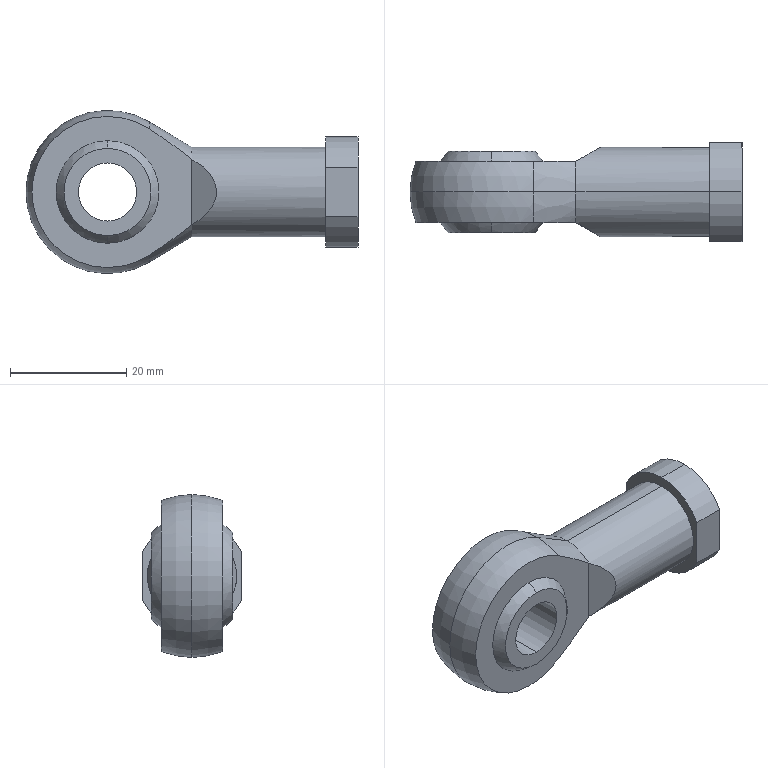Part | SolidWorks | features Draft 2, HoleWzd 2, ICE 2, BaseBody 1, Chamfer 1 | 1 solid | 32 faces | box 57 x 17 x 28 mm | volume 10383 mm3 | plane 10 | cylinder 9 | cone 7 | sphere 6 | commonest cylinder face diameters 19 x3 8.376 x2 10 x2 15.352 x2
STEP:
#1=CARTESIAN_POINT('',(42.188,0.,4.188));
#2=VERTEX_POINT('',#1);
#3=CARTESIAN_POINT('',(42.188,0.,-4.188));
#4=VERTEX_POINT('',#3);
#5=CARTESIAN_POINT('',(42.188,0.,0.));
#6=DIRECTION('',(1.,0.,0.));
#7=DIRECTION('',(0.,0.,1.));
#8=AXIS2_PLACEMENT_3D('',#5,#6,#7);
#9=CIRCLE('',#8,4.188);
#10=EDGE_CURVE('',#2,#4,#9,.T.);
#11=ORIENTED_EDGE('',*,*,#10,.F.);
#12=CARTESIAN_POINT('',(43.,0.,5.));
#13=VERTEX_POINT('',#12);
#14=CARTESIAN_POINT('',(42.188,0.,4.188));
#15=DIRECTION('',(0.7071,0.,0.7071));
#16=VECTOR('',#15,1000.);
#17=LINE('',#14,#16);
#18=EDGE_CURVE('',#2,#13,#17,.T.);
#19=ORIENTED_EDGE('',*,*,#18,.T.);
#20=CARTESIAN_POINT('',(43.,0.,-5.));
#21=VERTEX_POINT('',#20);
#22=CARTESIAN_POINT('',(43.,0.,0.));
#23=DIRECTION('',(-1.,0.,0.));
#24=DIRECTION('',(0.,0.,1.));
#25=AXIS2_PLACEMENT_3D('',#22,#23,#24);
#26=CIRCLE('',#25,5.);
#27=EDGE_CURVE('',#21,#13,#26,.T.);
#28=ORIENTED_EDGE('',*,*,#27,.F.);
#29=CARTESIAN_POINT('',(42.188,0.,-4.188));
#30=DIRECTION('',(0.7071,0.,-0.7071));
#31=VECTOR('',#30,1000.);
#32=LINE('',#29,#31);
#33=EDGE_CURVE('',#4,#21,#32,.T.);
#34=ORIENTED_EDGE('',*,*,#33,.F.);
#35=EDGE_LOOP('',(#11,#19,#28,#34));
#36=FACE_OUTER_BOUND('',#35,.T.);
#37=CARTESIAN_POINT('',(42.188,0.,0.));
#38=DIRECTION('',(1.,0.,0.));
#39=DIRECTION('',(0.,0.,-1.));
#40=AXIS2_PLACEMENT_3D('',#37,#38,#39);
#41=CONICAL_SURFACE('',#40,4.188,0.7854);
#42=ADVANCED_FACE('',(#36),#41,.F.);
#43=CARTESIAN_POINT('',(18.,0.,4.188));
#44=VERTEX_POINT('',#43);
#45=CARTESIAN_POINT('',(18.,0.,-4.188));
#46=VERTEX_POINT('',#45);
#47=CARTESIAN_POINT('',(18.,0.,0.));
#48=DIRECTION('',(1.,0.,0.));
#49=DIRECTION('',(0.,0.,-1.));
#50=AXIS2_PLACEMENT_3D('',#47,#48,#49);
#51=CIRCLE('',#50,4.188);
#52=EDGE_CURVE('',#44,#46,#51,.T.);
#53=ORIENTED_EDGE('',*,*,#52,.F.);
#54=CARTESIAN_POINT('',(43.,0.,4.188));
#55=DIRECTION('',(1.,0.,0.));
#56=VECTOR('',#55,1000.);
#57=LINE('',#54,#56);
#58=EDGE_CURVE('',#44,#2,#57,.T.);
#59=ORIENTED_EDGE('',*,*,#58,.T.);
#60=ORIENTED_EDGE('',*,*,#10,.T.);
#61=CARTESIAN_POINT('',(43.,0.,-4.188));
#62=DIRECTION('',(1.,0.,0.));
#63=VECTOR('',#62,1000.);
#64=LINE('',#61,#63);
#65=EDGE_CURVE('',#46,#4,#64,.T.);
#66=ORIENTED_EDGE('',*,*,#65,.F.);
#67=EDGE_LOOP('',(#53,#59,#60,#66));
#68=FACE_OUTER_BOUND('',#67,.T.);
#69=CARTESIAN_POINT('',(43.,0.,0.));
#70=DIRECTION('',(1.,0.,0.));
#71=DIRECTION('',(0.,0.,-1.));
#72=AXIS2_PLACEMENT_3D('',#69,#70,#71);
#73=CYLINDRICAL_SURFACE('',#72,4.188);
#74=ADVANCED_FACE('',(#68),#73,.F.);
#75=CARTESIAN_POINT('',(15.582,0.,0.));
#76=VERTEX_POINT('',#75);
#77=CARTESIAN_POINT('',(18.,0.,-4.188));
#78=DIRECTION('',(0.5,0.,-0.866));
#79=VECTOR('',#78,1000.);
#80=LINE('',#77,#79);
#81=EDGE_CURVE('',#76,#46,#80,.T.);
#82=ORIENTED_EDGE('',*,*,#81,.F.);
#83=CARTESIAN_POINT('',(18.,0.,4.188));
#84=DIRECTION('',(0.5,0.,0.866));
#85=VECTOR('',#84,1000.);
#86=LINE('',#83,#85);
#87=EDGE_CURVE('',#76,#44,#86,.T.);
#88=ORIENTED_EDGE('',*,*,#87,.T.);
#89=ORIENTED_EDGE('',*,*,#52,.T.);
#90=EDGE_LOOP('',(#82,#88,#89));
#91=FACE_OUTER_BOUND('',#90,.T.);
#92=CARTESIAN_POINT('',(18.,0.,0.));
#93=DIRECTION('',(1.,0.,0.));
#94=DIRECTION('',(0.,0.,-1.));
#95=AXIS2_PLACEMENT_3D('',#92,#93,#94);
#96=CONICAL_SURFACE('',#95,4.188,1.047);
#97=ADVANCED_FACE('',(#91),#96,.F.);
#98=CARTESIAN_POINT('',(0.,7.,-5.));
#99=VERTEX_POINT('',#98);
#100=CARTESIAN_POINT('',(0.,7.,5.));
#101=VERTEX_POINT('',#100);
#102=CARTESIAN_POINT('',(0.,7.,0.));
#103=DIRECTION('',(0.,1.,0.));
#104=DIRECTION('',(0.,0.,1.));
#105=AXIS2_PLACEMENT_3D('',#102,#103,#104);
#106=CIRCLE('',#105,5.);
#107=EDGE_CURVE('',#99,#101,#106,.T.);
#108=ORIENTED_EDGE('',*,*,#107,.T.);
#109=CARTESIAN_POINT('',(0.,-7.,5.));
#110=VERTEX_POINT('',#109);
#111=CARTESIAN_POINT('',(0.,-7.,5.));
#112=DIRECTION('',(0.,-1.,0.));
#113=VECTOR('',#112,1000.);
#114=LINE('',#111,#113);
#115=EDGE_CURVE('',#101,#110,#114,.T.);
#116=ORIENTED_EDGE('',*,*,#115,.T.);
#117=CARTESIAN_POINT('',(0.,-7.,-5.));
#118=VERTEX_POINT('',#117);
#119=CARTESIAN_POINT('',(0.,-7.,0.));
#120=DIRECTION('',(0.,-1.,0.));
#121=DIRECTION('',(0.,0.,-1.));
#122=AXIS2_PLACEMENT_3D('',#119,#120,#121);
#123=CIRCLE('',#122,5.);
#124=EDGE_CURVE('',#110,#118,#123,.T.);
#125=ORIENTED_EDGE('',*,*,#124,.T.);
#126=CARTESIAN_POINT('',(0.,-7.,-5.));
#127=DIRECTION('',(0.,-1.,0.));
#128=VECTOR('',#127,1000.);
#129=LINE('',#126,#128);
#130=EDGE_CURVE('',#99,#118,#129,.T.);
#131=ORIENTED_EDGE('',*,*,#130,.F.);
#132=EDGE_LOOP('',(#108,#116,#125,#131));
#133=FACE_OUTER_BOUND('',#132,.T.);
#134=CARTESIAN_POINT('',(0.,-7.,0.));
#135=DIRECTION('',(0.,-1.,0.));
#136=DIRECTION('',(0.,0.,-1.));
#137=AXIS2_PLACEMENT_3D('',#134,#135,#136);
#138=CYLINDRICAL_SURFACE('',#137,5.);
#139=ADVANCED_FACE('',(#133),#138,.F.);
#140=CARTESIAN_POINT('',(43.,-8.5,4.243));
#141=VERTEX_POINT('',#140);
#142=CARTESIAN_POINT('',(43.,0.,9.5));
#143=VERTEX_POINT('',#142);
#144=CARTESIAN_POINT('',(43.,0.,0.));
#145=DIRECTION('',(-1.,0.,0.));
#146=DIRECTION('',(0.,0.,1.));
#147=AXIS2_PLACEMENT_3D('',#144,#145,#146);
#148=CIRCLE('',#147,9.5);
#149=EDGE_CURVE('',#141,#143,#148,.T.);
#150=ORIENTED_EDGE('',*,*,#149,.T.);
#151=CARTESIAN_POINT('',(37.453,0.,9.5));
#152=VERTEX_POINT('',#151);
#153=CARTESIAN_POINT('',(43.,0.,9.5));
#154=DIRECTION('',(-1.,0.,0.));
#155=VECTOR('',#154,1000.);
#156=LINE('',#153,#155);
#157=EDGE_CURVE('',#143,#152,#156,.T.);
#158=ORIENTED_EDGE('',*,*,#157,.T.);
#159=CARTESIAN_POINT('',(37.453,-8.5,4.243));
#160=VERTEX_POINT('',#159);
#161=CARTESIAN_POINT('',(37.453,0.,0.));
#162=DIRECTION('',(-1.,0.,0.));
#163=DIRECTION('',(0.,0.,1.));
#164=AXIS2_PLACEMENT_3D('',#161,#162,#163);
#165=CIRCLE('',#164,9.5);
#166=EDGE_CURVE('',#160,#152,#165,.T.);
#167=ORIENTED_EDGE('',*,*,#166,.F.);
#168=CARTESIAN_POINT('',(43.,-8.5,4.243));
#169=DIRECTION('',(-1.,0.,0.));
#170=VECTOR('',#169,1000.);
#171=LINE('',#168,#170);
#172=EDGE_CURVE('',#141,#160,#171,.T.);
#173=ORIENTED_EDGE('',*,*,#172,.F.);
#174=EDGE_LOOP('',(#150,#158,#167,#173));
#175=FACE_OUTER_BOUND('',#174,.T.);
#176=CARTESIAN_POINT('',(43.,0.,0.));
#177=DIRECTION('',(-1.,0.,0.));
#178=DIRECTION('',(0.,0.,1.));
#179=AXIS2_PLACEMENT_3D('',#176,#177,#178);
#180=CYLINDRICAL_SURFACE('',#179,9.5);
#181=ADVANCED_FACE('',(#175),#180,.T.);
#182=CARTESIAN_POINT('',(37.453,0.,-7.676));
#183=VERTEX_POINT('',#182);
#184=CARTESIAN_POINT('',(37.453,0.,7.676));
#185=VERTEX_POINT('',#184);
#186=CARTESIAN_POINT('',(37.453,0.,0.));
#187=DIRECTION('',(1.,0.,0.));
#188=DIRECTION('',(0.,0.,-1.));
#189=AXIS2_PLACEMENT_3D('',#186,#187,#188);
#190=CIRCLE('',#189,7.676);
#191=EDGE_CURVE('',#183,#185,#190,.T.);
#192=ORIENTED_EDGE('',*,*,#191,.F.);
#193=CARTESIAN_POINT('',(14.491,0.,-7.676));
#194=VERTEX_POINT('',#193);
#195=CARTESIAN_POINT('',(37.453,0.,-7.676));
#196=DIRECTION('',(-1.,0.,0.));
#197=VECTOR('',#196,1000.);
#198=LINE('',#195,#197);
#199=EDGE_CURVE('',#183,#194,#198,.T.);
#200=ORIENTED_EDGE('',*,*,#199,.T.);
#201=CARTESIAN_POINT('',(14.491,5.25,-5.6));
#202=VERTEX_POINT('',#201);
#203=CARTESIAN_POINT('',(14.491,0.,0.));
#204=DIRECTION('',(1.,0.,0.));
#205=DIRECTION('',(0.,0.,1.));
#206=AXIS2_PLACEMENT_3D('',#203,#204,#205);
#207=CIRCLE('',#206,7.676);
#208=EDGE_CURVE('',#194,#202,#207,.T.);
#209=ORIENTED_EDGE('',*,*,#208,.T.);
#210=CARTESIAN_POINT('',(14.491,5.25,5.6));
#211=VERTEX_POINT('',#210);
#212=CARTESIAN_POINT('',(14.491,5.25,-5.6));
#213=CARTESIAN_POINT('',(20.468,8.701,-2.365));
#214=CARTESIAN_POINT('',(20.468,8.701,2.365));
#215=CARTESIAN_POINT('',(14.491,5.25,5.6));
#216=(BOUNDED_CURVE()B_SPLINE_CURVE(3,(#212,#213,#214,#215),.UNSPECIFIED.,.F.,.F.)B_SPLINE_CURVE_WITH_KNOTS((4,4),(2.324,3.959),.UNSPECIFIED.)CURVE()GEOMETRIC_REPRESENTATION_ITEM()RATIONAL_B_SPLINE_CURVE((1.,0.7893,0.7893,1.))REPRESENTATION_ITEM(''));
#217=EDGE_CURVE('',#202,#211,#216,.T.);
#218=ORIENTED_EDGE('',*,*,#217,.T.);
#219=CARTESIAN_POINT('',(14.491,0.,7.676));
#220=VERTEX_POINT('',#219);
#221=CARTESIAN_POINT('',(14.491,0.,0.));
#222=DIRECTION('',(1.,0.,0.));
#223=DIRECTION('',(0.,0.,1.));
#224=AXIS2_PLACEMENT_3D('',#221,#222,#223);
#225=CIRCLE('',#224,7.676);
#226=EDGE_CURVE('',#211,#220,#225,.T.);
#227=ORIENTED_EDGE('',*,*,#226,.T.);
#228=CARTESIAN_POINT('',(37.453,0.,7.676));
#229=DIRECTION('',(-1.,0.,0.));
#230=VECTOR('',#229,1000.);
#231=LINE('',#228,#230);
#232=EDGE_CURVE('',#185,#220,#231,.T.);
#233=ORIENTED_EDGE('',*,*,#232,.F.);
#234=EDGE_LOOP('',(#192,#200,#209,#218,#227,#233));
#235=FACE_OUTER_BOUND('',#234,.T.);
#236=CARTESIAN_POINT('',(37.453,0.,0.));
#237=DIRECTION('',(-1.,0.,0.));
#238=DIRECTION('',(0.,0.,1.));
#239=AXIS2_PLACEMENT_3D('',#236,#237,#238);
#240=CYLINDRICAL_SURFACE('',#239,7.676);
#241=ADVANCED_FACE('',(#235),#240,.T.);
#242=CARTESIAN_POINT('',(0.,5.25,-8.813));
#243=VERTEX_POINT('',#242);
#244=CARTESIAN_POINT('',(0.,5.25,8.813));
#245=VERTEX_POINT('',#244);
#246=CARTESIAN_POINT('',(0.,5.25,0.));
#247=DIRECTION('',(0.,1.,0.));
#248=DIRECTION('',(0.,0.,1.));
#249=AXIS2_PLACEMENT_3D('',#246,#247,#248);
#250=CIRCLE('',#249,8.813);
#251=EDGE_CURVE('',#243,#245,#250,.T.);
#252=ORIENTED_EDGE('',*,*,#251,.T.);
#253=CARTESIAN_POINT('',(0.,7.,7.498));
#254=VERTEX_POINT('',#253);
#255=CARTESIAN_POINT('',(0.,0.,0.));
#256=DIRECTION('',(-1.,0.,0.));
#257=DIRECTION('',(0.,0.,1.));
#258=AXIS2_PLACEMENT_3D('',#255,#256,#257);
#259=CIRCLE('',#258,10.258);
#260=EDGE_CURVE('',#245,#254,#259,.T.);
#261=ORIENTED_EDGE('',*,*,#260,.T.);
#262=CARTESIAN_POINT('',(0.,7.,-7.498));
#263=VERTEX_POINT('',#262);
#264=CARTESIAN_POINT('',(0.,7.,0.));
#265=DIRECTION('',(0.,-1.,0.));
#266=DIRECTION('',(0.,0.,1.));
#267=AXIS2_PLACEMENT_3D('',#264,#265,#266);
#268=CIRCLE('',#267,7.498);
#269=EDGE_CURVE('',#254,#263,#268,.T.);
#270=ORIENTED_EDGE('',*,*,#269,.T.);
#271=CARTESIAN_POINT('',(0.,0.,0.));
#272=DIRECTION('',(1.,0.,0.));
#273=DIRECTION('',(0.,1.,0.));
#274=AXIS2_PLACEMENT_3D('',#271,#272,#273);
#275=CIRCLE('',#274,10.258);
#276=EDGE_CURVE('',#243,#263,#275,.T.);
#277=ORIENTED_EDGE('',*,*,#276,.F.);
#278=EDGE_LOOP('',(#252,#261,#270,#277));
#279=FACE_OUTER_BOUND('',#278,.T.);
#280=CARTESIAN_POINT('',(0.,0.,0.));
#281=DIRECTION('',(-1.,0.,0.));
#282=DIRECTION('',(0.,0.5011,-0.8654));
#283=AXIS2_PLACEMENT_3D('',#280,#281,#282);
#284=SPHERICAL_SURFACE('',#283,10.258);
#285=ADVANCED_FACE('',(#279),#284,.T.);
#286=CARTESIAN_POINT('',(0.,-5.25,8.813));
#287=VERTEX_POINT('',#286);
#288=CARTESIAN_POINT('',(0.,-5.25,-8.813));
#289=VERTEX_POINT('',#288);
#290=CARTESIAN_POINT('',(0.,-5.25,0.));
#291=DIRECTION('',(0.,-1.,0.));
#292=DIRECTION('',(0.,0.,-1.));
#293=AXIS2_PLACEMENT_3D('',#290,#291,#292);
#294=CIRCLE('',#293,8.813);
#295=EDGE_CURVE('',#287,#289,#294,.T.);
#296=ORIENTED_EDGE('',*,*,#295,.T.);
#297=CARTESIAN_POINT('',(0.,-7.,-7.498));
#298=VERTEX_POINT('',#297);
#299=CARTESIAN_POINT('',(0.,0.,0.));
#300=DIRECTION('',(-1.,0.,0.));
#301=DIRECTION('',(0.,0.,1.));
#302=AXIS2_PLACEMENT_3D('',#299,#300,#301);
#303=CIRCLE('',#302,10.258);
#304=EDGE_CURVE('',#289,#298,#303,.T.);
#305=ORIENTED_EDGE('',*,*,#304,.T.);
#306=CARTESIAN_POINT('',(0.,-7.,7.498));
#307=VERTEX_POINT('',#306);
#308=CARTESIAN_POINT('',(0.,-7.,0.));
#309=DIRECTION('',(0.,1.,0.));
#310=DIRECTION('',(0.,0.,-1.));
#311=AXIS2_PLACEMENT_3D('',#308,#309,#310);
#312=CIRCLE('',#311,7.498);
#313=EDGE_CURVE('',#298,#307,#312,.T.);
#314=ORIENTED_EDGE('',*,*,#313,.T.);
#315=CARTESIAN_POINT('',(0.,0.,0.));
#316=DIRECTION('',(1.,0.,0.));
#317=DIRECTION('',(0.,1.,0.));
#318=AXIS2_PLACEMENT_3D('',#315,#316,#317);
#319=CIRCLE('',#318,10.258);
#320=EDGE_CURVE('',#287,#307,#319,.T.);
#321=ORIENTED_EDGE('',*,*,#320,.F.);
#322=EDGE_LOOP('',(#296,#305,#314,#321));
#323=FACE_OUTER_BOUND('',#322,.T.);
#324=CARTESIAN_POINT('',(0.,0.,0.));
#325=DIRECTION('',(-1.,0.,0.));
#326=DIRECTION('',(0.,-0.5011,0.8654));
#327=AXIS2_PLACEMENT_3D('',#324,#325,#326);
#328=SPHERICAL_SURFACE('',#327,10.258);
#329=ADVANCED_FACE('',(#323),#328,.T.);
#330=CARTESIAN_POINT('',(14.491,-5.25,5.6));
#331=VERTEX_POINT('',#330);
#332=CARTESIAN_POINT('',(14.491,0.,0.));
#333=DIRECTION('',(1.,0.,0.));
#334=DIRECTION('',(0.,0.,1.));
#335=AXIS2_PLACEMENT_3D('',#332,#333,#334);
#336=CIRCLE('',#335,7.676);
#337=EDGE_CURVE('',#220,#331,#336,.T.);
#338=ORIENTED_EDGE('',*,*,#337,.F.);
#339=CARTESIAN_POINT('',(7.15,0.,12.037));
#340=VERTEX_POINT('',#339);
#341=CARTESIAN_POINT('',(7.15,0.,12.037));
#342=DIRECTION('',(-0.8598,0.,0.5107));
#343=VECTOR('',#342,1000.);
#344=LINE('',#341,#343);
#345=EDGE_CURVE('',#220,#340,#344,.T.);
#346=ORIENTED_EDGE('',*,*,#345,.T.);
#347=CARTESIAN_POINT('',(7.15,-5.25,10.831));
#348=VERTEX_POINT('',#347);
#349=CARTESIAN_POINT('',(7.15,0.,0.));
#350=DIRECTION('',(1.,0.,0.));
#351=DIRECTION('',(0.,0.,1.));
#352=AXIS2_PLACEMENT_3D('',#349,#350,#351);
#353=CIRCLE('',#352,12.037);
#354=EDGE_CURVE('',#340,#348,#353,.T.);
#355=ORIENTED_EDGE('',*,*,#354,.T.);
#356=CARTESIAN_POINT('',(7.15,-5.25,10.831));
#357=CARTESIAN_POINT('',(7.848,-5.25,10.37));
#358=CARTESIAN_POINT('',(8.508,-5.25,9.929));
#359=CARTESIAN_POINT('',(9.441,-5.25,9.296));
#360=CARTESIAN_POINT('',(9.742,-5.25,9.09));
#361=CARTESIAN_POINT('',(10.18,-5.25,8.788));
#362=CARTESIAN_POINT('',(10.395,-5.25,8.639));
#363=CARTESIAN_POINT('',(10.64,-5.25,8.468));
#364=CARTESIAN_POINT('',(10.761,-5.25,8.384));
#365=CARTESIAN_POINT('',(10.821,-5.25,8.342));
#366=CARTESIAN_POINT('',(10.85,-5.25,8.321));
#367=CARTESIAN_POINT('',(10.863,-5.25,8.312));
#368=CARTESIAN_POINT('',(10.872,-5.25,8.306));
#369=CARTESIAN_POINT('',(10.875,-5.25,8.303));
#370=CARTESIAN_POINT('',(11.553,-5.25,7.827));
#371=CARTESIAN_POINT('',(12.177,-5.25,7.377));
#372=CARTESIAN_POINT('',(12.894,-5.25,6.843));
#373=CARTESIAN_POINT('',(13.07,-5.25,6.711));
#374=CARTESIAN_POINT('',(13.249,-5.25,6.575));
#375=CARTESIAN_POINT('',(13.292,-5.25,6.542));
#376=CARTESIAN_POINT('',(13.309,-5.25,6.53));
#377=CARTESIAN_POINT('',(13.338,-5.25,6.507));
#378=CARTESIAN_POINT('',(13.446,-5.25,6.425));
#379=CARTESIAN_POINT('',(13.852,-5.25,6.112));
#380=CARTESIAN_POINT('',(14.215,-5.25,5.824));
#381=CARTESIAN_POINT('',(14.491,-5.25,5.6));
#382=B_SPLINE_CURVE_WITH_KNOTS('',3,(#356,#357,#358,#359,#360,#361,#362,#363,#364,#365,#366,#367,#368,#369,#370,#371,#372,#373,#374,#375,#376,#377,#378,#379,#380,#381),.UNSPECIFIED.,.F.,.F.,(4,2,2,1,1,1,1,1,2,2,2,1,1,2,1,1,1,4),(0.,0.25,0.375,0.4375,0.4688,0.4844,0.4922,0.4961,0.498,0.5,0.75,0.8125,0.8281,0.832,0.8359,0.8437,0.875,1.),.UNSPECIFIED.);
#383=EDGE_CURVE('',#348,#331,#382,.T.);
#384=ORIENTED_EDGE('',*,*,#383,.T.);
#385=EDGE_LOOP('',(#338,#346,#355,#384));
#386=FACE_OUTER_BOUND('',#385,.T.);
#387=CARTESIAN_POINT('',(7.15,0.,0.));
#388=DIRECTION('',(-1.,0.,0.));
#389=DIRECTION('',(0.,0.,1.));
#390=AXIS2_PLACEMENT_3D('',#387,#388,#389);
#391=CONICAL_SURFACE('',#390,12.037,0.536);
#392=ADVANCED_FACE('',(#386),#391,.T.);
#393=CARTESIAN_POINT('',(-14.,0.,0.));
#394=VERTEX_POINT('',#393);
#395=CARTESIAN_POINT('',(0.,0.,0.));
#396=DIRECTION('',(0.,1.,0.));
#397=DIRECTION('',(0.,0.,1.));
#398=AXIS2_PLACEMENT_3D('',#395,#396,#397);
#399=CIRCLE('',#398,14.);
#400=EDGE_CURVE('',#394,#340,#399,.T.);
#401=ORIENTED_EDGE('',*,*,#400,.F.);
#402=CARTESIAN_POINT('',(7.15,0.,-12.037));
#403=VERTEX_POINT('',#402);
#404=CARTESIAN_POINT('',(0.,0.,0.));
#405=DIRECTION('',(0.,-1.,0.));
#406=DIRECTION('',(0.,0.,-1.));
#407=AXIS2_PLACEMENT_3D('',#404,#405,#406);
#408=CIRCLE('',#407,14.);
#409=EDGE_CURVE('',#394,#403,#408,.T.);
#410=ORIENTED_EDGE('',*,*,#409,.T.);
#411=CARTESIAN_POINT('',(7.15,-5.25,-10.831));
#412=VERTEX_POINT('',#411);
#413=CARTESIAN_POINT('',(7.15,0.,0.));
#414=DIRECTION('',(1.,0.,0.));
#415=DIRECTION('',(0.,-1.,0.));
#416=AXIS2_PLACEMENT_3D('',#413,#414,#415);
#417=CIRCLE('',#416,12.037);
#418=EDGE_CURVE('',#412,#403,#417,.T.);
#419=ORIENTED_EDGE('',*,*,#418,.F.);
#420=CARTESIAN_POINT('',(0.,-5.25,0.));
#421=DIRECTION('',(0.,1.,0.));
#422=DIRECTION('',(0.,0.,1.));
#423=AXIS2_PLACEMENT_3D('',#420,#421,#422);
#424=CIRCLE('',#423,12.978);
#425=EDGE_CURVE('',#412,#348,#424,.T.);
#426=ORIENTED_EDGE('',*,*,#425,.T.);
#427=ORIENTED_EDGE('',*,*,#354,.F.);
#428=EDGE_LOOP('',(#401,#410,#419,#426,#427));
#429=FACE_OUTER_BOUND('',#428,.T.);
#430=CARTESIAN_POINT('',(0.,0.,0.));
#431=DIRECTION('',(0.,-1.,0.));
#432=DIRECTION('',(0.,0.,1.));
#433=AXIS2_PLACEMENT_3D('',#430,#431,#432);
#434=SPHERICAL_SURFACE('',#433,14.);
#435=ADVANCED_FACE('',(#429),#434,.T.);
#436=ORIENTED_EDGE('',*,*,#295,.F.);
#437=CARTESIAN_POINT('',(0.,-5.25,0.));
#438=DIRECTION('',(0.,-1.,0.));
#439=DIRECTION('',(0.,0.,-1.));
#440=AXIS2_PLACEMENT_3D('',#437,#438,#439);
#441=CIRCLE('',#440,8.813);
#442=EDGE_CURVE('',#289,#287,#441,.T.);
#443=ORIENTED_EDGE('',*,*,#442,.F.);
#444=EDGE_LOOP('',(#436,#443));
#445=FACE_BOUND('',#444,.T.);
#446=CARTESIAN_POINT('',(14.491,-5.25,-5.6));
#447=VERTEX_POINT('',#446);
#448=CARTESIAN_POINT('',(14.491,-5.25,-5.6));
#449=CARTESIAN_POINT('',(14.215,-5.25,-5.824));
#450=CARTESIAN_POINT('',(13.925,-5.25,-6.055));
#451=CARTESIAN_POINT('',(13.543,-5.25,-6.35));
#452=CARTESIAN_POINT('',(13.446,-5.25,-6.425));
#453=CARTESIAN_POINT('',(13.348,-5.25,-6.499));
#454=CARTESIAN_POINT('',(13.318,-5.25,-6.522));
#455=CARTESIAN_POINT('',(13.309,-5.25,-6.53));
#456=CARTESIAN_POINT('',(13.292,-5.25,-6.542));
#457=CARTESIAN_POINT('',(13.249,-5.25,-6.575));
#458=CARTESIAN_POINT('',(13.07,-5.25,-6.711));
#459=CARTESIAN_POINT('',(12.894,-5.25,-6.843));
#460=CARTESIAN_POINT('',(12.464,-5.25,-7.163));
#461=CARTESIAN_POINT('',(12.164,-5.25,-7.382));
#462=CARTESIAN_POINT('',(11.697,-5.25,-7.72));
#463=CARTESIAN_POINT('',(11.458,-5.25,-7.891));
#464=CARTESIAN_POINT('',(11.172,-5.25,-8.094));
#465=CARTESIAN_POINT('',(11.027,-5.25,-8.197));
#466=CARTESIAN_POINT('',(10.954,-5.25,-8.248));
#467=CARTESIAN_POINT('',(10.917,-5.25,-8.274));
#468=CARTESIAN_POINT('',(10.901,-5.25,-8.285));
#469=CARTESIAN_POINT('',(10.891,-5.25,-8.292));
#470=CARTESIAN_POINT('',(10.885,-5.25,-8.297));
#471=CARTESIAN_POINT('',(9.79,-5.25,-9.066));
#472=CARTESIAN_POINT('',(8.547,-5.25,-9.909));
#473=CARTESIAN_POINT('',(7.15,-5.25,-10.831));
#474=B_SPLINE_CURVE_WITH_KNOTS('',3,(#448,#449,#450,#451,#452,#453,#454,#455,#456,#457,#458,#459,#460,#461,#462,#463,#464,#465,#466,#467,#468,#469,#470,#471,#472,#473),.UNSPECIFIED.,.F.,.F.,(4,2,1,2,2,1,1,2,2,1,1,1,1,1,2,2,4),(0.,0.125,0.1563,0.1641,0.168,0.1719,0.1875,0.25,0.375,0.4375,0.4688,0.4844,0.4922,0.4961,0.498,0.5,1.),.UNSPECIFIED.);
#475=EDGE_CURVE('',#447,#412,#474,.T.);
#476=ORIENTED_EDGE('',*,*,#475,.F.);
#477=CARTESIAN_POINT('',(14.491,-5.25,14.));
#478=DIRECTION('',(0.,0.,-1.));
#479=VECTOR('',#478,1000.);
#480=LINE('',#477,#479);
#481=EDGE_CURVE('',#331,#447,#480,.T.);
#482=ORIENTED_EDGE('',*,*,#481,.F.);
#483=ORIENTED_EDGE('',*,*,#383,.F.);
#484=ORIENTED_EDGE('',*,*,#425,.F.);
#485=EDGE_LOOP('',(#476,#482,#483,#484));
#486=FACE_OUTER_BOUND('',#485,.T.);
#487=CARTESIAN_POINT('',(14.491,-5.25,14.));
#488=DIRECTION('',(0.,-1.,0.));
#489=DIRECTION('',(0.,0.,-1.));
#490=AXIS2_PLACEMENT_3D('',#487,#488,#489);
#491=PLANE('',#490);
#492=ADVANCED_FACE('',(#445,#486),#491,.T.);
#493=ORIENTED_EDGE('',*,*,#251,.F.);
#494=CARTESIAN_POINT('',(0.,5.25,0.));
#495=DIRECTION('',(0.,1.,0.));
#496=DIRECTION('',(0.,0.,1.));
#497=AXIS2_PLACEMENT_3D('',#494,#495,#496);
#498=CIRCLE('',#497,8.813);
#499=EDGE_CURVE('',#245,#243,#498,.T.);
#500=ORIENTED_EDGE('',*,*,#499,.F.);
#501=EDGE_LOOP('',(#493,#500));
#502=FACE_BOUND('',#501,.T.);
#503=CARTESIAN_POINT('',(7.15,5.25,10.831));
#504=VERTEX_POINT('',#503);
#505=CARTESIAN_POINT('',(14.491,5.25,5.6));
#506=CARTESIAN_POINT('',(14.215,5.25,5.824));
#507=CARTESIAN_POINT('',(13.925,5.25,6.055));
#508=CARTESIAN_POINT('',(13.543,5.25,6.35));
#509=CARTESIAN_POINT('',(13.446,5.25,6.425));
#510=CARTESIAN_POINT('',(13.348,5.25,6.499));
#511=CARTESIAN_POINT('',(13.318,5.25,6.522));
#512=CARTESIAN_POINT('',(13.309,5.25,6.53));
#513=CARTESIAN_POINT('',(13.292,5.25,6.542));
#514=CARTESIAN_POINT('',(13.249,5.25,6.575));
#515=CARTESIAN_POINT('',(13.07,5.25,6.711));
#516=CARTESIAN_POINT('',(12.894,5.25,6.843));
#517=CARTESIAN_POINT('',(12.464,5.25,7.163));
#518=CARTESIAN_POINT('',(12.164,5.25,7.382));
#519=CARTESIAN_POINT('',(11.697,5.25,7.72));
#520=CARTESIAN_POINT('',(11.458,5.25,7.891));
#521=CARTESIAN_POINT('',(11.172,5.25,8.094));
#522=CARTESIAN_POINT('',(11.027,5.25,8.197));
#523=CARTESIAN_POINT('',(10.954,5.25,8.248));
#524=CARTESIAN_POINT('',(10.917,5.25,8.274));
#525=CARTESIAN_POINT('',(10.901,5.25,8.285));
#526=CARTESIAN_POINT('',(10.891,5.25,8.292));
#527=CARTESIAN_POINT('',(10.885,5.25,8.297));
#528=CARTESIAN_POINT('',(9.79,5.25,9.066));
#529=CARTESIAN_POINT('',(8.547,5.25,9.909));
#530=CARTESIAN_POINT('',(7.15,5.25,10.831));
#531=B_SPLINE_CURVE_WITH_KNOTS('',3,(#505,#506,#507,#508,#509,#510,#511,#512,#513,#514,#515,#516,#517,#518,#519,#520,#521,#522,#523,#524,#525,#526,#527,#528,#529,#530),.UNSPECIFIED.,.F.,.F.,(4,2,1,2,2,1,1,2,2,1,1,1,1,1,2,2,4),(0.,0.125,0.1563,0.1641,0.168,0.1719,0.1875,0.25,0.375,0.4375,0.4688,0.4844,0.4922,0.4961,0.498,0.5,1.),.UNSPECIFIED.);
#532=EDGE_CURVE('',#211,#504,#531,.T.);
#533=ORIENTED_EDGE('',*,*,#532,.F.);
#534=CARTESIAN_POINT('',(14.491,5.25,14.));
#535=DIRECTION('',(0.,0.,1.));
#536=VECTOR('',#535,1000.);
#537=LINE('',#534,#536);
#538=EDGE_CURVE('',#202,#211,#537,.T.);
#539=ORIENTED_EDGE('',*,*,#538,.F.);
#540=CARTESIAN_POINT('',(7.15,5.25,-10.831));
#541=VERTEX_POINT('',#540);
#542=CARTESIAN_POINT('',(7.15,5.25,-10.831));
#543=CARTESIAN_POINT('',(7.848,5.25,-10.37));
#544=CARTESIAN_POINT('',(8.508,5.25,-9.929));
#545=CARTESIAN_POINT('',(9.441,5.25,-9.296));
#546=CARTESIAN_POINT('',(9.742,5.25,-9.09));
#547=CARTESIAN_POINT('',(10.18,5.25,-8.788));
#548=CARTESIAN_POINT('',(10.395,5.25,-8.639));
#549=CARTESIAN_POINT('',(10.64,5.25,-8.468));
#550=CARTESIAN_POINT('',(10.761,5.25,-8.384));
#551=CARTESIAN_POINT('',(10.821,5.25,-8.342));
#552=CARTESIAN_POINT('',(10.85,5.25,-8.321));
#553=CARTESIAN_POINT('',(10.863,5.25,-8.312));
#554=CARTESIAN_POINT('',(10.872,5.25,-8.306));
#555=CARTESIAN_POINT('',(10.875,5.25,-8.303));
#556=CARTESIAN_POINT('',(11.553,5.25,-7.827));
#557=CARTESIAN_POINT('',(12.177,5.25,-7.377));
#558=CARTESIAN_POINT('',(12.894,5.25,-6.843));
#559=CARTESIAN_POINT('',(13.07,5.25,-6.711));
#560=CARTESIAN_POINT('',(13.249,5.25,-6.575));
#561=CARTESIAN_POINT('',(13.292,5.25,-6.542));
#562=CARTESIAN_POINT('',(13.309,5.25,-6.53));
#563=CARTESIAN_POINT('',(13.338,5.25,-6.507));
#564=CARTESIAN_POINT('',(13.446,5.25,-6.425));
#565=CARTESIAN_POINT('',(13.852,5.25,-6.112));
#566=CARTESIAN_POINT('',(14.215,5.25,-5.824));
#567=CARTESIAN_POINT('',(14.491,5.25,-5.6));
#568=B_SPLINE_CURVE_WITH_KNOTS('',3,(#542,#543,#544,#545,#546,#547,#548,#549,#550,#551,#552,#553,#554,#555,#556,#557,#558,#559,#560,#561,#562,#563,#564,#565,#566,#567),.UNSPECIFIED.,.F.,.F.,(4,2,2,1,1,1,1,1,2,2,2,1,1,2,1,1,1,4),(0.,0.25,0.375,0.4375,0.4687,0.4844,0.4922,0.4961,0.498,0.5,0.75,0.8125,0.8281,0.832,0.8359,0.8437,0.875,1.),.UNSPECIFIED.);
#569=EDGE_CURVE('',#541,#202,#568,.T.);
#570=ORIENTED_EDGE('',*,*,#569,.F.);
#571=CARTESIAN_POINT('',(0.,5.25,0.));
#572=DIRECTION('',(0.,-1.,0.));
#573=DIRECTION('',(0.,0.,1.));
#574=AXIS2_PLACEMENT_3D('',#571,#572,#573);
#575=CIRCLE('',#574,12.978);
#576=EDGE_CURVE('',#504,#541,#575,.T.);
#577=ORIENTED_EDGE('',*,*,#576,.F.);
#578=EDGE_LOOP('',(#533,#539,#570,#577));
#579=FACE_OUTER_BOUND('',#578,.T.);
#580=CARTESIAN_POINT('',(-19.,5.25,14.));
#581=DIRECTION('',(0.,1.,0.));
#582=DIRECTION('',(1.,0.,0.));
#583=AXIS2_PLACEMENT_3D('',#580,#581,#582);
#584=PLANE('',#583);
#585=ADVANCED_FACE('',(#502,#579),#584,.T.);
#586=ORIENTED_EDGE('',*,*,#475,.T.);
#587=ORIENTED_EDGE('',*,*,#418,.T.);
#588=CARTESIAN_POINT('',(7.15,0.,0.));
#589=DIRECTION('',(1.,0.,0.));
#590=DIRECTION('',(0.,-1.,0.));
#591=AXIS2_PLACEMENT_3D('',#588,#589,#590);
#592=CIRCLE('',#591,12.037);
#593=EDGE_CURVE('',#403,#541,#592,.T.);
#594=ORIENTED_EDGE('',*,*,#593,.T.);
#595=ORIENTED_EDGE('',*,*,#569,.T.);
#596=ORIENTED_EDGE('',*,*,#208,.F.);
#597=CARTESIAN_POINT('',(14.491,0.,0.));
#598=DIRECTION('',(1.,0.,0.));
#599=DIRECTION('',(0.,0.,1.));
#600=AXIS2_PLACEMENT_3D('',#597,#598,#599);
#601=CIRCLE('',#600,7.676);
#602=EDGE_CURVE('',#447,#194,#601,.T.);
#603=ORIENTED_EDGE('',*,*,#602,.F.);
#604=EDGE_LOOP('',(#586,#587,#594,#595,#596,#603));
#605=FACE_OUTER_BOUND('',#604,.T.);
#606=CARTESIAN_POINT('',(7.15,0.,0.));
#607=DIRECTION('',(-1.,0.,0.));
#608=DIRECTION('',(0.,-1.,0.));
#609=AXIS2_PLACEMENT_3D('',#606,#607,#608);
#610=CONICAL_SURFACE('',#609,12.037,0.536);
#611=ADVANCED_FACE('',(#605),#610,.T.);
#612=ORIENTED_EDGE('',*,*,#409,.F.);
#613=ORIENTED_EDGE('',*,*,#400,.T.);
#614=CARTESIAN_POINT('',(7.15,0.,0.));
#615=DIRECTION('',(1.,0.,0.));
#616=DIRECTION('',(0.,0.,1.));
#617=AXIS2_PLACEMENT_3D('',#614,#615,#616);
#618=CIRCLE('',#617,12.037);
#619=EDGE_CURVE('',#504,#340,#618,.T.);
#620=ORIENTED_EDGE('',*,*,#619,.F.);
#621=ORIENTED_EDGE('',*,*,#576,.T.);
#622=ORIENTED_EDGE('',*,*,#593,.F.);
#623=EDGE_LOOP('',(#612,#613,#620,#621,#622));
#624=FACE_OUTER_BOUND('',#623,.T.);
#625=CARTESIAN_POINT('',(0.,0.,0.));
#626=DIRECTION('',(0.,-1.,0.));
#627=DIRECTION('',(0.,0.,1.));
#628=AXIS2_PLACEMENT_3D('',#625,#626,#627);
#629=SPHERICAL_SURFACE('',#628,14.);
#630=ADVANCED_FACE('',(#624),#629,.T.);
#631=ORIENTED_EDGE('',*,*,#345,.F.);
#632=ORIENTED_EDGE('',*,*,#226,.F.);
#633=ORIENTED_EDGE('',*,*,#532,.T.);
#634=ORIENTED_EDGE('',*,*,#619,.T.);
#635=EDGE_LOOP('',(#631,#632,#633,#634));
#636=FACE_OUTER_BOUND('',#635,.T.);
#637=CARTESIAN_POINT('',(7.15,0.,0.));
#638=DIRECTION('',(-1.,0.,0.));
#639=DIRECTION('',(0.,0.,1.));
#640=AXIS2_PLACEMENT_3D('',#637,#638,#639);
#641=CONICAL_SURFACE('',#640,12.037,0.536);
#642=ADVANCED_FACE('',(#636),#641,.T.);
#643=ORIENTED_EDGE('',*,*,#304,.F.);
#644=ORIENTED_EDGE('',*,*,#442,.T.);
#645=ORIENTED_EDGE('',*,*,#320,.T.);
#646=CARTESIAN_POINT('',(0.,-7.,0.));
#647=DIRECTION('',(0.,1.,0.));
#648=DIRECTION('',(0.,0.,-1.));
#649=AXIS2_PLACEMENT_3D('',#646,#647,#648);
#650=CIRCLE('',#649,7.498);
#651=EDGE_CURVE('',#307,#298,#650,.T.);
#652=ORIENTED_EDGE('',*,*,#651,.T.);
#653=EDGE_LOOP('',(#643,#644,#645,#652));
#654=FACE_OUTER_BOUND('',#653,.T.);
#655=CARTESIAN_POINT('',(0.,0.,0.));
#656=DIRECTION('',(-1.,0.,0.));
#657=DIRECTION('',(0.,-0.5011,0.8654));
#658=AXIS2_PLACEMENT_3D('',#655,#656,#657);
#659=SPHERICAL_SURFACE('',#658,10.258);
#660=ADVANCED_FACE('',(#654),#659,.T.);
#661=CARTESIAN_POINT('',(0.,-7.,0.));
#662=DIRECTION('',(0.,-1.,0.));
#663=DIRECTION('',(0.,0.,-1.));
#664=AXIS2_PLACEMENT_3D('',#661,#662,#663);
#665=CIRCLE('',#664,5.);
#666=EDGE_CURVE('',#118,#110,#665,.T.);
#667=ORIENTED_EDGE('',*,*,#666,.F.);
#668=ORIENTED_EDGE('',*,*,#124,.F.);
#669=EDGE_LOOP('',(#667,#668));
#670=FACE_BOUND('',#669,.T.);
#671=ORIENTED_EDGE('',*,*,#651,.F.);
#672=ORIENTED_EDGE('',*,*,#313,.F.);
#673=EDGE_LOOP('',(#671,#672));
#674=FACE_OUTER_BOUND('',#673,.T.);
#675=CARTESIAN_POINT('',(5.,-7.,0.));
#676=DIRECTION('',(0.,-1.,0.));
#677=DIRECTION('',(0.,0.,-1.));
#678=AXIS2_PLACEMENT_3D('',#675,#676,#677);
#679=PLANE('',#678);
#680=ADVANCED_FACE('',(#670,#674),#679,.T.);
#681=ORIENTED_EDGE('',*,*,#260,.F.);
#682=ORIENTED_EDGE('',*,*,#499,.T.);
#683=ORIENTED_EDGE('',*,*,#276,.T.);
#684=CARTESIAN_POINT('',(0.,7.,0.));
#685=DIRECTION('',(0.,-1.,0.));
#686=DIRECTION('',(0.,0.,1.));
#687=AXIS2_PLACEMENT_3D('',#684,#685,#686);
#688=CIRCLE('',#687,7.498);
#689=EDGE_CURVE('',#263,#254,#688,.T.);
#690=ORIENTED_EDGE('',*,*,#689,.T.);
#691=EDGE_LOOP('',(#681,#682,#683,#690));
#692=FACE_OUTER_BOUND('',#691,.T.);
#693=CARTESIAN_POINT('',(0.,0.,0.));
#694=DIRECTION('',(-1.,0.,0.));
#695=DIRECTION('',(0.,0.5011,-0.8654));
#696=AXIS2_PLACEMENT_3D('',#693,#694,#695);
#697=SPHERICAL_SURFACE('',#696,10.258);
#698=ADVANCED_FACE('',(#692),#697,.T.);
#699=ORIENTED_EDGE('',*,*,#107,.F.);
#700=CARTESIAN_POINT('',(0.,7.,0.));
#701=DIRECTION('',(0.,1.,0.));
#702=DIRECTION('',(0.,0.,1.));
#703=AXIS2_PLACEMENT_3D('',#700,#701,#702);
#704=CIRCLE('',#703,5.);
#705=EDGE_CURVE('',#101,#99,#704,.T.);
#706=ORIENTED_EDGE('',*,*,#705,.F.);
#707=EDGE_LOOP('',(#699,#706));
#708=FACE_BOUND('',#707,.T.);
#709=ORIENTED_EDGE('',*,*,#689,.F.);
#710=ORIENTED_EDGE('',*,*,#269,.F.);
#711=EDGE_LOOP('',(#709,#710));
#712=FACE_OUTER_BOUND('',#711,.T.);
#713=CARTESIAN_POINT('',(7.498,7.,0.));
#714=DIRECTION('',(0.,1.,0.));
#715=DIRECTION('',(1.,0.,0.));
#716=AXIS2_PLACEMENT_3D('',#713,#714,#715);
#717=PLANE('',#716);
#718=ADVANCED_FACE('',(#708,#712),#717,.T.);
#719=CARTESIAN_POINT('',(14.491,-5.25,5.6));
#720=CARTESIAN_POINT('',(20.468,-8.701,2.365));
#721=CARTESIAN_POINT('',(20.468,-8.701,-2.365));
#722=CARTESIAN_POINT('',(14.491,-5.25,-5.6));
#723=(BOUNDED_CURVE()B_SPLINE_CURVE(3,(#719,#720,#721,#722),.UNSPECIFIED.,.F.,.F.)B_SPLINE_CURVE_WITH_KNOTS((4,4),(2.324,3.959),.UNSPECIFIED.)CURVE()GEOMETRIC_REPRESENTATION_ITEM()RATIONAL_B_SPLINE_CURVE((1.,0.7893,0.7893,1.))REPRESENTATION_ITEM(''));
#724=EDGE_CURVE('',#331,#447,#723,.T.);
#725=ORIENTED_EDGE('',*,*,#724,.F.);
#726=ORIENTED_EDGE('',*,*,#481,.T.);
#727=EDGE_LOOP('',(#725,#726));
#728=FACE_OUTER_BOUND('',#727,.T.);
#729=CARTESIAN_POINT('',(14.491,-5.25,14.));
#730=DIRECTION('',(-0.5,-0.866,0.));
#731=DIRECTION('',(0.866,-0.5,0.));
#732=AXIS2_PLACEMENT_3D('',#729,#730,#731);
#733=PLANE('',#732);
#734=ADVANCED_FACE('',(#728),#733,.T.);
#735=ORIENTED_EDGE('',*,*,#217,.F.);
#736=ORIENTED_EDGE('',*,*,#538,.T.);
#737=EDGE_LOOP('',(#735,#736));
#738=FACE_OUTER_BOUND('',#737,.T.);
#739=CARTESIAN_POINT('',(14.491,5.25,14.));
#740=DIRECTION('',(-0.5,0.866,0.));
#741=DIRECTION('',(-0.866,-0.5,0.));
#742=AXIS2_PLACEMENT_3D('',#739,#740,#741);
#743=PLANE('',#742);
#744=ADVANCED_FACE('',(#738),#743,.T.);
#745=ORIENTED_EDGE('',*,*,#199,.F.);
#746=CARTESIAN_POINT('',(37.453,0.,0.));
#747=DIRECTION('',(1.,0.,0.));
#748=DIRECTION('',(0.,0.,-1.));
#749=AXIS2_PLACEMENT_3D('',#746,#747,#748);
#750=CIRCLE('',#749,7.676);
#751=EDGE_CURVE('',#185,#183,#750,.T.);
#752=ORIENTED_EDGE('',*,*,#751,.F.);
#753=ORIENTED_EDGE('',*,*,#232,.T.);
#754=ORIENTED_EDGE('',*,*,#337,.T.);
#755=ORIENTED_EDGE('',*,*,#724,.T.);
#756=ORIENTED_EDGE('',*,*,#602,.T.);
#757=EDGE_LOOP('',(#745,#752,#753,#754,#755,#756));
#758=FACE_OUTER_BOUND('',#757,.T.);
#759=CARTESIAN_POINT('',(37.453,0.,0.));
#760=DIRECTION('',(-1.,0.,0.));
#761=DIRECTION('',(0.,0.,1.));
#762=AXIS2_PLACEMENT_3D('',#759,#760,#761);
#763=CYLINDRICAL_SURFACE('',#762,7.676);
#764=ADVANCED_FACE('',(#758),#763,.T.);
#765=CARTESIAN_POINT('',(37.453,8.5,-4.243));
#766=VERTEX_POINT('',#765);
#767=CARTESIAN_POINT('',(37.453,-8.5,-4.243));
#768=VERTEX_POINT('',#767);
#769=CARTESIAN_POINT('',(37.453,0.,0.));
#770=DIRECTION('',(-1.,0.,0.));
#771=DIRECTION('',(0.,0.,1.));
#772=AXIS2_PLACEMENT_3D('',#769,#770,#771);
#773=CIRCLE('',#772,9.5);
#774=EDGE_CURVE('',#766,#768,#773,.T.);
#775=ORIENTED_EDGE('',*,*,#774,.F.);
#776=CARTESIAN_POINT('',(43.,8.5,-4.243));
#777=VERTEX_POINT('',#776);
#778=CARTESIAN_POINT('',(43.,8.5,-4.243));
#779=DIRECTION('',(-1.,0.,0.));
#780=VECTOR('',#779,1000.);
#781=LINE('',#778,#780);
#782=EDGE_CURVE('',#777,#766,#781,.T.);
#783=ORIENTED_EDGE('',*,*,#782,.F.);
#784=CARTESIAN_POINT('',(43.,-8.5,-4.243));
#785=VERTEX_POINT('',#784);
#786=CARTESIAN_POINT('',(43.,0.,0.));
#787=DIRECTION('',(-1.,0.,0.));
#788=DIRECTION('',(0.,0.,1.));
#789=AXIS2_PLACEMENT_3D('',#786,#787,#788);
#790=CIRCLE('',#789,9.5);
#791=EDGE_CURVE('',#777,#785,#790,.T.);
#792=ORIENTED_EDGE('',*,*,#791,.T.);
#793=CARTESIAN_POINT('',(43.,-8.5,-4.243));
#794=DIRECTION('',(-1.,0.,0.));
#795=VECTOR('',#794,1000.);
#796=LINE('',#793,#795);
#797=EDGE_CURVE('',#785,#768,#796,.T.);
#798=ORIENTED_EDGE('',*,*,#797,.T.);
#799=EDGE_LOOP('',(#775,#783,#792,#798));
#800=FACE_OUTER_BOUND('',#799,.T.);
#801=CARTESIAN_POINT('',(43.,0.,0.));
#802=DIRECTION('',(-1.,0.,0.));
#803=DIRECTION('',(0.,0.,1.));
#804=AXIS2_PLACEMENT_3D('',#801,#802,#803);
#805=CYLINDRICAL_SURFACE('',#804,9.5);
#806=ADVANCED_FACE('',(#800),#805,.T.);
#807=CARTESIAN_POINT('',(37.453,8.5,4.243));
#808=VERTEX_POINT('',#807);
#809=CARTESIAN_POINT('',(37.453,8.5,4.243));
#810=DIRECTION('',(0.,0.,-1.));
#811=VECTOR('',#810,1000.);
#812=LINE('',#809,#811);
#813=EDGE_CURVE('',#808,#766,#812,.T.);
#814=ORIENTED_EDGE('',*,*,#813,.F.);
#815=CARTESIAN_POINT('',(43.,8.5,4.243));
#816=VERTEX_POINT('',#815);
#817=CARTESIAN_POINT('',(43.,8.5,4.243));
#818=DIRECTION('',(-1.,0.,0.));
#819=VECTOR('',#818,1000.);
#820=LINE('',#817,#819);
#821=EDGE_CURVE('',#816,#808,#820,.T.);
#822=ORIENTED_EDGE('',*,*,#821,.F.);
#823=CARTESIAN_POINT('',(43.,8.5,4.243));
#824=DIRECTION('',(0.,0.,-1.));
#825=VECTOR('',#824,1000.);
#826=LINE('',#823,#825);
#827=EDGE_CURVE('',#816,#777,#826,.T.);
#828=ORIENTED_EDGE('',*,*,#827,.T.);
#829=ORIENTED_EDGE('',*,*,#782,.T.);
#830=EDGE_LOOP('',(#814,#822,#828,#829));
#831=FACE_OUTER_BOUND('',#830,.T.);
#832=CARTESIAN_POINT('',(43.,8.5,4.243));
#833=DIRECTION('',(0.,1.,0.));
#834=DIRECTION('',(0.,0.,1.));
#835=AXIS2_PLACEMENT_3D('',#832,#833,#834);
#836=PLANE('',#835);
#837=ADVANCED_FACE('',(#831),#836,.T.);
#838=ORIENTED_EDGE('',*,*,#157,.F.);
#839=CARTESIAN_POINT('',(43.,0.,0.));
#840=DIRECTION('',(-1.,0.,0.));
#841=DIRECTION('',(0.,0.,1.));
#842=AXIS2_PLACEMENT_3D('',#839,#840,#841);
#843=CIRCLE('',#842,9.5);
#844=EDGE_CURVE('',#143,#816,#843,.T.);
#845=ORIENTED_EDGE('',*,*,#844,.T.);
#846=ORIENTED_EDGE('',*,*,#821,.T.);
#847=CARTESIAN_POINT('',(37.453,0.,0.));
#848=DIRECTION('',(-1.,0.,0.));
#849=DIRECTION('',(0.,0.,1.));
#850=AXIS2_PLACEMENT_3D('',#847,#848,#849);
#851=CIRCLE('',#850,9.5);
#852=EDGE_CURVE('',#152,#808,#851,.T.);
#853=ORIENTED_EDGE('',*,*,#852,.F.);
#854=EDGE_LOOP('',(#838,#845,#846,#853));
#855=FACE_OUTER_BOUND('',#854,.T.);
#856=CARTESIAN_POINT('',(43.,0.,0.));
#857=DIRECTION('',(-1.,0.,0.));
#858=DIRECTION('',(0.,0.,1.));
#859=AXIS2_PLACEMENT_3D('',#856,#857,#858);
#860=CYLINDRICAL_SURFACE('',#859,9.5);
#861=ADVANCED_FACE('',(#855),#860,.T.);
#862=CARTESIAN_POINT('',(37.453,-8.5,-4.243));
#863=DIRECTION('',(0.,0.,1.));
#864=VECTOR('',#863,1000.);
#865=LINE('',#862,#864);
#866=EDGE_CURVE('',#768,#160,#865,.T.);
#867=ORIENTED_EDGE('',*,*,#866,.F.);
#868=ORIENTED_EDGE('',*,*,#797,.F.);
#869=CARTESIAN_POINT('',(43.,-8.5,-4.243));
#870=DIRECTION('',(0.,0.,1.));
#871=VECTOR('',#870,1000.);
#872=LINE('',#869,#871);
#873=EDGE_CURVE('',#785,#141,#872,.T.);
#874=ORIENTED_EDGE('',*,*,#873,.T.);
#875=ORIENTED_EDGE('',*,*,#172,.T.);
#876=EDGE_LOOP('',(#867,#868,#874,#875));
#877=FACE_OUTER_BOUND('',#876,.T.);
#878=CARTESIAN_POINT('',(43.,-8.5,-4.243));
#879=DIRECTION('',(0.,-1.,0.));
#880=DIRECTION('',(0.,0.,-1.));
#881=AXIS2_PLACEMENT_3D('',#878,#879,#880);
#882=PLANE('',#881);
#883=ADVANCED_FACE('',(#877),#882,.T.);
#884=ORIENTED_EDGE('',*,*,#27,.T.);
#885=CARTESIAN_POINT('',(43.,0.,0.));
#886=DIRECTION('',(-1.,0.,0.));
#887=DIRECTION('',(0.,0.,1.));
#888=AXIS2_PLACEMENT_3D('',#885,#886,#887);
#889=CIRCLE('',#888,5.);
#890=EDGE_CURVE('',#13,#21,#889,.T.);
#891=ORIENTED_EDGE('',*,*,#890,.T.);
#892=EDGE_LOOP('',(#884,#891));
#893=FACE_BOUND('',#892,.T.);
#894=ORIENTED_EDGE('',*,*,#791,.F.);
#895=ORIENTED_EDGE('',*,*,#827,.F.);
#896=ORIENTED_EDGE('',*,*,#844,.F.);
#897=ORIENTED_EDGE('',*,*,#149,.F.);
#898=ORIENTED_EDGE('',*,*,#873,.F.);
#899=EDGE_LOOP('',(#894,#895,#896,#897,#898));
#900=FACE_OUTER_BOUND('',#899,.T.);
#901=CARTESIAN_POINT('',(43.,0.,0.));
#902=DIRECTION('',(-1.,0.,0.));
#903=DIRECTION('',(0.,0.,1.));
#904=AXIS2_PLACEMENT_3D('',#901,#902,#903);
#905=PLANE('',#904);
#906=ADVANCED_FACE('',(#893,#900),#905,.F.);
#907=ORIENTED_EDGE('',*,*,#751,.T.);
#908=ORIENTED_EDGE('',*,*,#191,.T.);
#909=EDGE_LOOP('',(#907,#908));
#910=FACE_BOUND('',#909,.T.);
#911=ORIENTED_EDGE('',*,*,#774,.T.);
#912=ORIENTED_EDGE('',*,*,#866,.T.);
#913=ORIENTED_EDGE('',*,*,#166,.T.);
#914=ORIENTED_EDGE('',*,*,#852,.T.);
#915=ORIENTED_EDGE('',*,*,#813,.T.);
#916=EDGE_LOOP('',(#911,#912,#913,#914,#915));
#917=FACE_OUTER_BOUND('',#916,.T.);
#918=CARTESIAN_POINT('',(37.453,0.,0.));
#919=DIRECTION('',(-1.,0.,0.));
#920=DIRECTION('',(0.,0.,1.));
#921=AXIS2_PLACEMENT_3D('',#918,#919,#920);
#922=PLANE('',#921);
#923=ADVANCED_FACE('',(#910,#917),#922,.T.);
#924=ORIENTED_EDGE('',*,*,#115,.F.);
#925=ORIENTED_EDGE('',*,*,#705,.T.);
#926=ORIENTED_EDGE('',*,*,#130,.T.);
#927=ORIENTED_EDGE('',*,*,#666,.T.);
#928=EDGE_LOOP('',(#924,#925,#926,#927));
#929=FACE_OUTER_BOUND('',#928,.T.);
#930=CARTESIAN_POINT('',(0.,-7.,0.));
#931=DIRECTION('',(0.,-1.,0.));
#932=DIRECTION('',(0.,0.,-1.));
#933=AXIS2_PLACEMENT_3D('',#930,#931,#932);
#934=CYLINDRICAL_SURFACE('',#933,5.);
#935=ADVANCED_FACE('',(#929),#934,.F.);
#936=ORIENTED_EDGE('',*,*,#87,.F.);
#937=ORIENTED_EDGE('',*,*,#81,.T.);
#938=CARTESIAN_POINT('',(18.,0.,0.));
#939=DIRECTION('',(1.,0.,0.));
#940=DIRECTION('',(0.,0.,-1.));
#941=AXIS2_PLACEMENT_3D('',#938,#939,#940);
#942=CIRCLE('',#941,4.188);
#943=EDGE_CURVE('',#46,#44,#942,.T.);
#944=ORIENTED_EDGE('',*,*,#943,.T.);
#945=EDGE_LOOP('',(#936,#937,#944));
#946=FACE_OUTER_BOUND('',#945,.T.);
#947=CARTESIAN_POINT('',(18.,0.,0.));
#948=DIRECTION('',(1.,0.,0.));
#949=DIRECTION('',(0.,0.,-1.));
#950=AXIS2_PLACEMENT_3D('',#947,#948,#949);
#951=CONICAL_SURFACE('',#950,4.188,1.047);
#952=ADVANCED_FACE('',(#946),#951,.F.);
#953=ORIENTED_EDGE('',*,*,#58,.F.);
#954=ORIENTED_EDGE('',*,*,#943,.F.);
#955=ORIENTED_EDGE('',*,*,#65,.T.);
#956=CARTESIAN_POINT('',(42.188,0.,0.));
#957=DIRECTION('',(1.,0.,0.));
#958=DIRECTION('',(0.,0.,1.));
#959=AXIS2_PLACEMENT_3D('',#956,#957,#958);
#960=CIRCLE('',#959,4.188);
#961=EDGE_CURVE('',#4,#2,#960,.T.);
#962=ORIENTED_EDGE('',*,*,#961,.T.);
#963=EDGE_LOOP('',(#953,#954,#955,#962));
#964=FACE_OUTER_BOUND('',#963,.T.);
#965=CARTESIAN_POINT('',(43.,0.,0.));
#966=DIRECTION('',(1.,0.,0.));
#967=DIRECTION('',(0.,0.,-1.));
#968=AXIS2_PLACEMENT_3D('',#965,#966,#967);
#969=CYLINDRICAL_SURFACE('',#968,4.188);
#970=ADVANCED_FACE('',(#964),#969,.F.);
#971=ORIENTED_EDGE('',*,*,#18,.F.);
#972=ORIENTED_EDGE('',*,*,#961,.F.);
#973=ORIENTED_EDGE('',*,*,#33,.T.);
#974=ORIENTED_EDGE('',*,*,#890,.F.);
#975=EDGE_LOOP('',(#971,#972,#973,#974));
#976=FACE_OUTER_BOUND('',#975,.T.);
#977=CARTESIAN_POINT('',(42.188,0.,0.));
#978=DIRECTION('',(1.,0.,0.));
#979=DIRECTION('',(0.,0.,-1.));
#980=AXIS2_PLACEMENT_3D('',#977,#978,#979);
#981=CONICAL_SURFACE('',#980,4.188,0.7854);
#982=ADVANCED_FACE('',(#976),#981,.F.);
#983=CLOSED_SHELL('',(#42,#74,#97,#139,#181,#241,#285,#329,#392,#435,#492,#585,#611,#630,#642,#660,#680,#698,#718,#734,#744,#764,#806,#837,#861,#883,#906,#923,#935,#952,#970,#982));
#984=MANIFOLD_SOLID_BREP('',#983);
#985=CARTESIAN_POINT('',(0.,0.,0.));
#986=DIRECTION('',(0.,0.,1.));
#987=DIRECTION('',(1.,0.,0.));
#988=AXIS2_PLACEMENT_3D('',#985,#986,#987);
#989=(LENGTH_UNIT()NAMED_UNIT(*)SI_UNIT(.MILLI.,.METRE.));
#990=UNCERTAINTY_MEASURE_WITH_UNIT(LENGTH_MEASURE(0.00001),#989,'','');
#991=(NAMED_UNIT(*)PLANE_ANGLE_UNIT()SI_UNIT($,.RADIAN.));
#992=(NAMED_UNIT(*)SI_UNIT($,.STERADIAN.)SOLID_ANGLE_UNIT());
#993=(GEOMETRIC_REPRESENTATION_CONTEXT(3)GLOBAL_UNCERTAINTY_ASSIGNED_CONTEXT((#990))GLOBAL_UNIT_ASSIGNED_CONTEXT((#989,#991,#992))REPRESENTATION_CONTEXT('',''));
#994=ADVANCED_BREP_SHAPE_REPRESENTATION('',(#984,#988),#993);